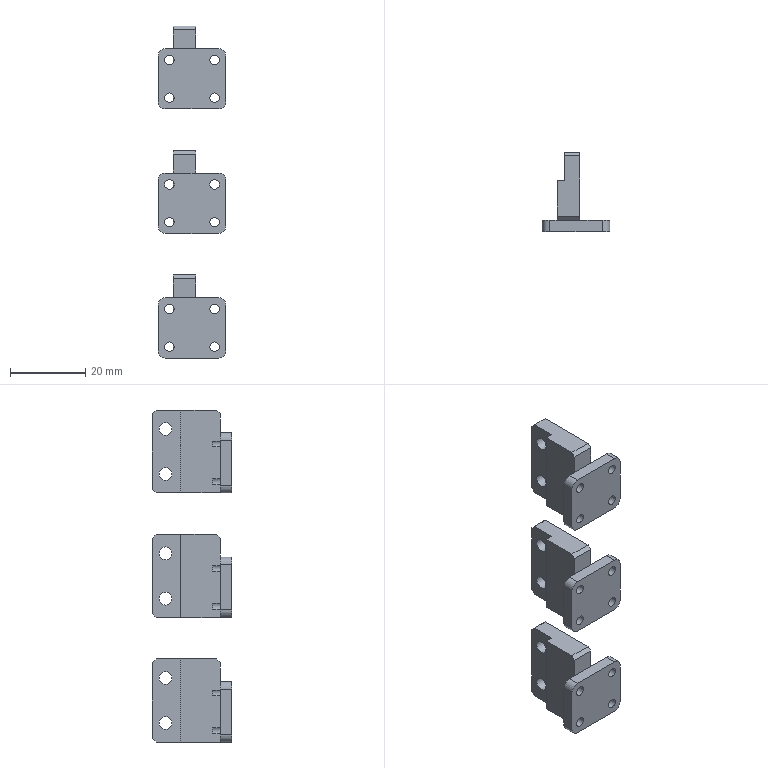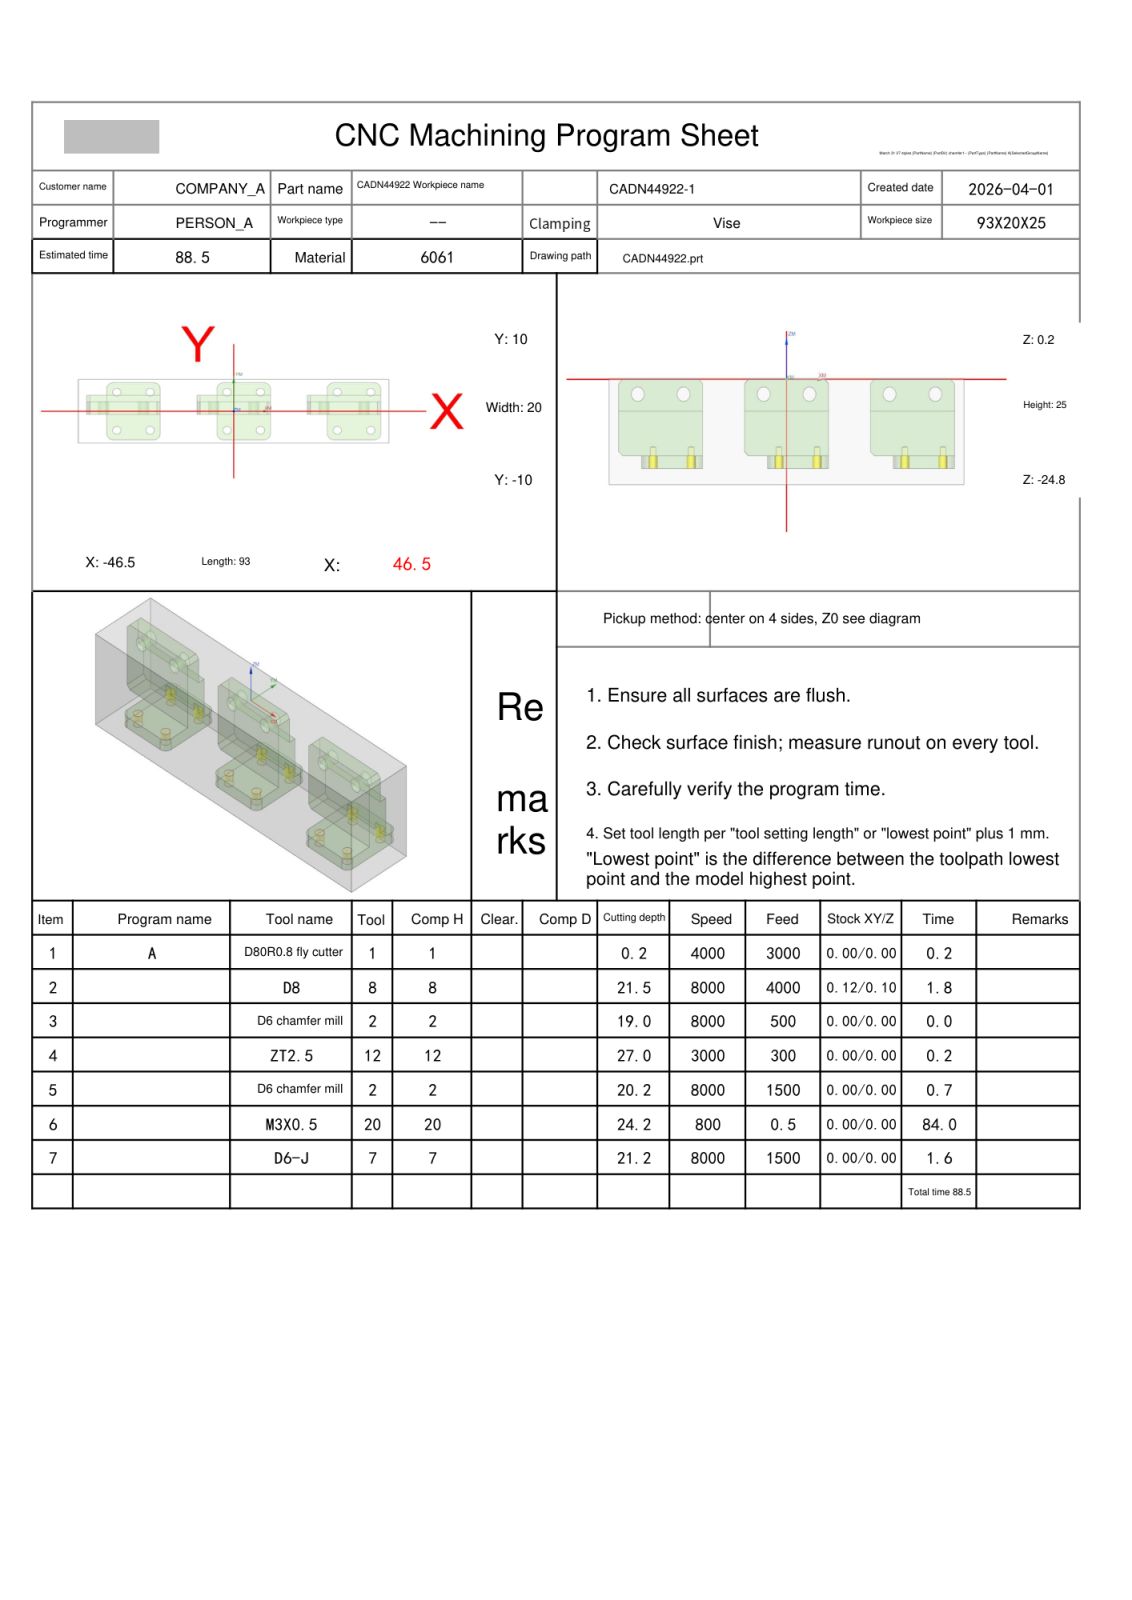NC program | NX | posted by the shop | part box 18 x 21 x 88 mm
Lines 3372 to 4142 of 4142:
N3 T02 M06
(D6 chamfer mill  D=6. R=0. H=02 ce=0.00 di=0.10)
G00 G90 G54 X-35. Y-6. M03 S8000
G43 H02 Z20.
M08
G98 G81 X-35. Y-6. Z-18.8 R-17. F500.
X-25.
X-2.
X8.
X31.
X41.
G80
G00 Z20.
G91 G28 Z0.0
M05
M09
G91 G28 Z0.0
M01
N4 T12 M06
(ZT2.5 D=2.5 DR_a=118 H=12)
G00 G90 G54 X-35. Y-6. M03 S3000
G43 H12 Z20.
M08
G98 G83 X-35. Y-6. Z-26.751 R-17. F300. Q2.
X-25.
X-2.
X8.
X31.
X41.
G80
G00 Z20.
G91 G28 Z0.0
M05
M09
G91 G28 Z0.0
M01
N5 T02 M06
(D6 chamfer mill  D=6. R=0. H=02 ce=0.00 di=0.10)
G00 G90 G54 X-35. Y-6. M03 S8000
G43 H02 Z20.
M08
G98 G81 X-35. Y-6. Z-19.75 R-15. F500.
X-25.
X-2.
X8.
X31.
X41.
G80
G00 Z20.
G00 G90 X-44.708 Y-3.9 M03 S6500
Z20.
Z-.2
G01 Z-1.7 F1500.
X-44.699 Y-3.832
X-44.7 Y-3.763
Y5.763
X-44.699 Y5.832
X-44.708 Y5.9
Z-.2
G00 Z20.
X-11.708 Y-3.9
Z-.2
G01 Z-1.7
X-11.699 Y-3.832
X-11.7 Y-3.763
Y5.763
X-11.699 Y5.832
X-11.708 Y5.9
Z-.2
G00 Z20.
X-21.292
Z-.2
G01 Z-1.7
X-21.301 Y5.832
X-21.3 Y5.763
Y-3.763
X-21.301 Y-3.832
X-21.292 Y-3.9
Z-.2
G00 Z20.
X21.292
Z-.2
G01 Z-1.7
X21.301 Y-3.832
X21.3 Y-3.763
Y5.763
X21.301 Y5.832
X21.292 Y5.9
Z-.2
G00 Z20.
X11.708
Z-.2
G01 Z-1.7
X11.699 Y5.832
X11.7 Y5.763
Y-3.763
X11.699 Y-3.832
X11.708 Y-3.9
Z-.2
G00 Z20.
X44.708 Y5.9
Z-.2
G01 Z-1.7
X44.699 Y5.832
X44.7 Y5.763
Y-3.763
X44.699 Y-3.832
X44.708 Y-3.9
Z-.2
G00 Z20.
G00 G90 X-43.604 Y4.689 M03 S6500
Z20.
Z2.
G01 Z-2. F1500.
X-43.351 Y4.765
X-43. Y4.8
X-23.
X-22.649 Y4.765
X-22.396 Y4.689
Z2.
G00 Y-2.689
G01 Z-2.
X-22.649 Y-2.765
X-23. Y-2.8
X-33.
X-43.
X-43.351 Y-2.765
X-43.604 Y-2.689
Z2.
G00 Z10.
X10.604
Z2.
G01 Z-2.
X10.351 Y-2.765
X10. Y-2.8
X-10.
X-10.351 Y-2.765
X-10.604 Y-2.689
Z2.
G00 Y4.689
G01 Z-2.
X-10.351 Y4.765
X-10. Y4.8
X0.0
X10.
X10.351 Y4.765
X10.604 Y4.689
Z2.
G00 Z10.
X43.604 Y-2.689
Z2.
G01 Z-2.
X43.351 Y-2.765
X43. Y-2.8
X23.
X22.649 Y-2.765
X22.396 Y-2.689
Z2.
G00 Y4.689
G01 Z-2.
X22.649 Y4.765
X23. Y4.8
X33.
X43.
X43.351 Y4.765
X43.604 Y4.689
Z2.
G00 Z10.
X20.059 Y5.65
Z-2.127
G01 Z-9.5
G03 X20.37 Y5.808 I-.745 J1.856
G01 X20.418 Y5.834
X20.441 Y5.883
X20.503 Y6.
G02 X22. Y6.8 I1.497 J-1.
G01 X23.375
X24.75
X27.5
X33.
X37.125
X39.875
X41.25
X44.
G02 X45.497 Y6. I0.0 J-1.8
G01 X45.559 Y5.883
X45.582 Y5.834
X45.63 Y5.808
G03 X45.941 Y5.65 I1.056 J1.698
G01 Z-2.127
G00 Z10.
X-12.941
Z-2.127
G01 Z-9.5
G03 X-12.63 Y5.808 I-.745 J1.856
G01 X-12.582 Y5.834
X-12.559 Y5.883
X-12.497 Y6.
G02 X-11. Y6.8 I1.497 J-1.
G01 X-9.625
X-8.25
X-5.5
X0.0
X4.125
X6.875
X8.25
X11.
G02 X12.497 Y6. I0.0 J-1.8
G01 X12.559 Y5.883
X12.582 Y5.834
X12.63 Y5.808
G03 X12.941 Y5.65 I1.056 J1.698
G01 Z-2.127
G00 Z10.
X-45.941
Z-2.127
G01 Z-9.5
G03 X-45.63 Y5.808 I-.745 J1.856
G01 X-45.582 Y5.834
X-45.559 Y5.883
X-45.497 Y6.
G02 X-44. Y6.8 I1.497 J-1.
G01 X-42.625
X-41.25
X-38.5
X-33.
X-28.875
X-26.125
X-24.75
X-22.
G02 X-20.503 Y6. I0.0 J-1.8
G01 X-20.441 Y5.883
X-20.418 Y5.834
X-20.37 Y5.808
G03 X-20.059 Y5.65 I1.056 J1.698
G01 Z-2.127
G00 Z10.
X-20.087 Y-3.573
Z-2.127
G01 Z-20.
X-20.148 Y-3.636
X-20.187 Y-3.716
X-20.206 Y-3.737
X-20.2 Y-3.766
Y-4.
Y-7.
G02 X-24. Y-10.8 I-3.8 J0.0
G01 X-31.5
X-33.
X-36.
G02 X-39.8 Y-7. I0.0 J3.8
G01 Y-4.281
X-39.805 Y-4.261
X-39.845 Y-4.204
Z-1.805
G00 Z10.
X-39.667 Y8.208
Z-9.31
G01 Z-20.
X-39.581 Y8.268
X-39.563 Y8.293
X-39.457 Y8.579
G02 X-36. Y10.8 I3.457 J-1.579
G01 X-24.
G02 X-20.354 Y8.071 I0.0 J-3.8
G01 X-20.296 Y7.806
X-20.289 Y7.757
X-20.254 Y7.723
G03 X-20.023 Y7.51 I1.332 J1.211
G01 Z-9.296
G00 Z10.
X12.913 Y-3.573
Z-2.127
G01 Z-20.
X12.852 Y-3.636
X12.813 Y-3.716
X12.794 Y-3.737
X12.8 Y-3.766
Y-7.
G02 X9. Y-10.8 I-3.8 J0.0
G01 X-3.
G02 X-6.8 Y-7. I0.0 J3.8
G01 Y-4.281
X-6.805 Y-4.261
X-6.845 Y-4.204
Z-1.805
G00 Z10.
X-6.667 Y8.208
Z-9.31
G01 Z-20.
X-6.581 Y8.268
X-6.563 Y8.293
X-6.457 Y8.579
G02 X-3. Y10.8 I3.457 J-1.579
G01 X9.
G02 X12.646 Y8.071 I0.0 J-3.8
G01 X12.704 Y7.806
X12.711 Y7.757
X12.746 Y7.723
G03 X12.977 Y7.51 I1.332 J1.211
G01 Z-9.296
G00 Z10.
X45.913 Y-3.573
Z-2.127
G01 Z-20.
X45.852 Y-3.636
X45.813 Y-3.716
X45.794 Y-3.737
X45.8 Y-3.766
Y-7.
G02 X42. Y-10.8 I-3.8 J0.0
G01 X30.
G02 X26.2 Y-7. I0.0 J3.8
G01 Y-4.281
X26.195 Y-4.261
X26.155 Y-4.204
Z-1.805
G00 Z10.
X26.333 Y8.208
Z-9.31
G01 Z-20.
X26.419 Y8.268
X26.437 Y8.293
X26.543 Y8.579
G02 X30. Y10.8 I3.457 J-1.579
G01 X42.
G02 X45.646 Y8.071 I0.0 J-3.8
G01 X45.704 Y7.806
X45.711 Y7.757
X45.746 Y7.723
G03 X45.977 Y7.51 I1.332 J1.211
G01 Z-9.296
G00 Z20.
G91 G28 Z0.0
M05
M09
G91 G28 Z0.0
M01
N6 T20 M06
(M3X0.5 D=2.5 DR_a=180 H=20)
G00 G90 G54 X-35. Y-6. M03 S800
G43 H20 Z20.
M08
G95
G98 G84 X-35. Y-6. Z-24. R-17. F.5 Q5.
X-25.
X-2.
X8.
X31.
X41.
G80
G94
G00 Z20.
G91 G28 Z0.0
M05
M09
G91 G28 Z0.0
M01
N7 T07 M06
(D6-J  D=6. R=0. H=07 ce=0.40 di=0.00)
G00 G90 G54 X-18.69 Y-10.2 M03 S7000
G43 H07 Z10.4
M08
Z-16.5
G01 Z-18. F1500.
G03 X-19.729 Y-9.6 I-1.039 J-.6
G01 X-39.919
G02 X-40.454 Y-9.273 I0.0 J.6
X-40.963 Y-7.605 I4.454 J2.273
G01 X-40.967 Y-7.54
G02 X-40.427 Y-7. I.54 J0.0
G01 X-19.54
G03 X-19. Y-6.46 I0.0 J.54
G01 Y-5.
G03 X-19.6 Y-4.4 I-.6 J0.0
G01 X-41.
G03 X-42.2 Y-5.6 I0.0 J-1.2
G01 Z-16.5
G00 Z-14.
X14.31 Y-10.2
Z-16.5
G01 Z-18.
G03 X13.271 Y-9.6 I-1.039 J-.6
G01 X-6.919
G02 X-7.454 Y-9.273 I0.0 J.6
X-7.963 Y-7.605 I4.454 J2.273
G01 X-7.967 Y-7.54
G02 X-7.427 Y-7. I.54 J0.0
G01 X13.46
G03 X14. Y-6.46 I0.0 J.54
G01 Y-5.
G03 X13.4 Y-4.4 I-.6 J0.0
G01 X-8.
G03 X-9.2 Y-5.6 I0.0 J-1.2
G01 Z-16.5
G00 Z-14.
X47.31 Y-10.2
Z-16.5
G01 Z-18.
G03 X46.271 Y-9.6 I-1.039 J-.6
G01 X26.08
G02 X25.547 Y-9.273 I0.0 J.6
X25.028 Y-7.531 I4.453 J2.273
G01 X25.026 Y-7.48
G02 X25.505 Y-7. I.48 J0.0
G01 X46.46
G03 X47. Y-6.46 I0.0 J.54
G01 Y-5.
G03 X46.4 Y-4.4 I-.6 J0.0
G01 X25.
G03 X23.8 Y-5.6 I0.0 J-1.2
G01 Z-16.5
G00 Z10.4
G00 G90 X21.083 Y6.995 M03 S8000
Z5.2
Z-4.25
G01 Z-5.25 F1000.
G41 D07
X21.106 Y6.796
G03 X22. Y6. I.894 J.104
G01 X44.
G02 X47. Y3. I0.0 J-3.
G01 Y-1.018
G02 X44. Y-4. I-3. J.018
G01 X22.
G02 X19. Y-1. I0.0 J3.
G01 Y3.
G02 X22. Y6. I3. J0.0
G03 X22.9 Y6.9 I0.0 J.9
G01 G40 Y7.1
Z-4.25
G00 Z5.2
X-44.917 Y6.995
Z-4.25
G01 Z-5.25
G41 D07
X-44.894 Y6.796
G03 X-44. Y6. I.894 J.104
G01 X-22.
G02 X-19. Y3. I0.0 J-3.
G01 Y-1.
X-19.001 Y-1.079
G02 X-22. Y-4. I-2.999 J.079
G01 X-44.
G02 X-47. Y-1. I0.0 J3.
G01 Y3.012
G02 X-44. Y6. I3. J-.012
G03 X-43.1 Y6.9 I0.0 J.9
G01 G40 Y7.1
Z-4.25
G00 Z5.2
X-11.917 Y6.995
Z-4.25
G01 Z-5.25
G41 D07
X-11.894 Y6.796
G03 X-11. Y6. I.894 J.104
G01 X11.
G02 X14. Y3. I0.0 J-3.
G01 Y-1.
X13.999 Y-1.078
G02 X11. Y-4. I-2.999 J.078
G01 X-11.
G02 X-14. Y-1. I0.0 J3.
G01 Y3.
G02 X-11. Y6. I3. J0.0
G03 X-10.1 Y6.9 I0.0 J.9
G01 G40 Y7.1
Z-4.25
G00 X-11.917 Y8.995
Z-9.5
G01 Z-10.5
G41 D07
X-11.894 Y8.796
G03 X-11. Y8. I.894 J.104
G01 X11.
G02 X13.999 Y5.077 I0.0 J-3.
G01 X14. Y5.
Y-1.
X13.999 Y-1.072
G02 X11. Y-4. I-2.999 J.072
G01 X-11.
G02 X-14. Y-1. I0.0 J3.
G01 Y5.
G02 X-11. Y8. I3. J0.0
G03 X-10.1 Y8.9 I0.0 J.9
G01 G40 Y9.1
Z-9.5
G00 Z3.
X-44.917 Y8.995
Z-9.5
G01 Z-10.5
G41 D07
X-44.894 Y8.796
G03 X-44. Y8. I.894 J.104
G01 X-22.
G02 X-19. Y5. I0.0 J-3.
G01 Y-1.
X-19.001 Y-1.079
G02 X-22. Y-4. I-2.999 J.079
G01 X-44.
G02 X-47. Y-1. I0.0 J3.
G01 Y5.
G02 X-44. Y8. I3. J0.0
G03 X-43.1 Y8.9 I0.0 J.9
G01 G40 Y9.1
Z-9.5
G00 X-44.917 Y8.995
Z-14.75
G01 Z-15.75
G41 D07
X-44.894 Y8.796
G03 X-44. Y8. I.894 J.104
G01 X-22.
G02 X-19. Y5. I0.0 J-3.
G01 Y-1.
X-19.001 Y-1.079
G02 X-22. Y-4. I-2.999 J.079
G01 X-44.
G02 X-47. Y-1. I0.0 J3.
G01 Y5.
G02 X-44. Y8. I3. J0.0
G03 X-43.1 Y8.9 I0.0 J.9
G01 G40 Y9.1
Z-14.75
G00 Z3.
X21.083 Y8.995
Z-9.5
G01 Z-10.5
G41 D07
X21.106 Y8.796
G03 X22. Y8. I.894 J.104
G01 X44.
G02 X47. Y5. I0.0 J-3.
G01 Y-1.014
G02 X44. Y-4. I-3. J.014
G01 X22.
G02 X19. Y-1. I0.0 J3.
G01 Y5.
G02 X22. Y8. I3. J0.0
G03 X22.9 Y8.9 I0.0 J.9
G01 G40 Y9.1
Z-9.5
G00 Z5.2
X-15.1 Y2.099
Z-6.5
G01 Z-7.5
G41 D07
X-14.9
G03 X-14. Y2.999 I0.0 J.9
G02 X-11. Y6. I3. J0.0
G01 X11.
G02 X14. Y3. I0.0 J-3.
G03 X14.9 Y2.099 I.9 J0.0
G01 G40 X15.1
Z-6.5
G00 Z5.2
X-48.1 Y2.104
Z-6.5
G01 Z-7.5
G41 D07
X-47.9
G03 X-47. Y2.999 I0.0 J.9
G01 Y3.031
G02 X-44. Y6. I3. J-.031
G01 X-22.
G02 X-19. Y3. I0.0 J-3.
G03 X-18.1 Y2.099 I.9 J0.0
G01 G40 X-17.9
Z-6.5
G00 Z5.2
X17.9 Y2.1
Z-6.5
G01 Z-7.5
G41 D07
X18.1
G03 X19. Y3. I0.0 J.9
G02 X22. Y6. I3. J0.0
G01 X44.
G02 X47. Y3. I0.0 J-3.
G03 X47.9 Y2.099 I.9 J0.0
G01 G40 X48.1
Z-6.5
G00 Z5.2
X21.083 Y8.995
Z-14.75
G01 Z-15.75
G41 D07
X21.106 Y8.796
G03 X22. Y8. I.894 J.104
G01 X44.
G02 X47. Y5. I0.0 J-3.
G01 Y-1.029
G02 X44. Y-4. I-3. J.029
G01 X22.
G02 X19. Y-1. I0.0 J3.
G01 Y5.
G02 X22. Y8. I3. J0.0
G03 X22.9 Y8.9 I0.0 J.9
G01 G40 Y9.1
Z-14.75
G00 Z5.2
X48.1 Y-.104
Z-17.
G01 Z-18.
G41 D07
X47.9
G03 X47. Y-.999 I0.0 J-.9
G01 Y-1.029
G02 X44. Y-4. I-3. J.029
G01 X25.
G03 X24.1 Y-4.9 I0.0 J-.9
G01 G40 Y-5.1
Z-17.
G00 Z5.2
X24.201 Y9.1
Z-17.
G01 Z-18.
G41 D07
Y8.9
G03 X25.101 Y8. I.9 J0.0
G01 X44.
G02 X47. Y5. I0.0 J-3.
G03 X47.9 Y4.099 I.9 J0.0
G01 G40 X48.1
Z-17.
G00 Z5.2
X-11.917 Y8.995
Z-14.75
G01 Z-15.75
G41 D07
X-11.894 Y8.796
G03 X-11. Y8. I.894 J.104
G01 X11.
G02 X14. Y5. I0.0 J-3.
G01 Y-1.
X13.999 Y-1.091
G02 X11. Y-4. I-2.999 J.091
G01 X-11.
G02 X-14. Y-1. I0.0 J3.
G01 Y5.
G02 X-11. Y8. I3. J0.0
G03 X-10.1 Y8.9 I0.0 J.9
G01 G40 Y9.1
Z-14.75
G00 Z5.2
X15.1 Y-.114
Z-17.
G01 Z-18.
G41 D07
X14.9
G03 X14. Y-1. I0.0 J-.9
G01 X13.999 Y-1.091
G02 X11. Y-4. I-2.999 J.091
G01 X-8.
G03 X-8.9 Y-4.9 I0.0 J-.9
G01 G40 Y-5.1
Z-17.
G00 Z5.2
X-8.799 Y9.1
Z-17.
G01 Z-18.
G41 D07
Y8.9
G03 X-7.899 Y8. I.9 J0.0
G01 X11.
G02 X14. Y5. I0.0 J-3.
G03 X14.9 Y4.1 I.9 J0.0
G01 G40 X15.1
Z-17.
G00 Z5.2
X-41.799 Y9.1
Z-17.
G01 Z-18.
G41 D07
Y8.9
G03 X-40.899 Y8. I.9 J0.0
G01 X-22.
G02 X-19. Y5. I0.0 J-3.
G03 X-18.1 Y4.099 I.9 J0.0
G01 G40 X-17.9
Z-17.
G00 Z5.2
Y-.111
Z-17.
G01 Z-18.
G41 D07
X-18.1
G03 X-19. Y-.999 I0.0 J-.9
G01 X-19.001 Y-1.079
G02 X-22. Y-4. I-2.999 J.079
G01 X-41.
G03 X-41.9 Y-4.9 I0.0 J-.9
G01 G40 Y-5.1
Z-17.
G00 Z5.2
X-3.913 Y13.031
Z-20.
G01 Z-21.
G41 D07
X-3.897 Y12.831
G03 X-3. Y12. I.897 J.069
G01 X9.
G02 X14. Y7. I0.0 J-5.
G01 Y-7.
G02 X9. Y-12. I-5. J0.0
G01 X-3.
G02 X-8. Y-7. I0.0 J5.
G01 Y-4.
X-11.
G02 X-14. Y-1. I0.0 J3.
G01 Y5.
G02 X-11. Y8. I3. J0.0
G01 X-7.899
G02 X-3. Y12. I4.899 J-1.
G03 X-2.1 Y12.9 I0.0 J.9
G01 G40 Y13.1
Z-20.
G00 Z-7.5
X-36.913 Y13.031
Z-20.
G01 Z-21.
G41 D07
X-36.897 Y12.831
G03 X-36. Y12. I.897 J.069
G01 X-24.
G02 X-19. Y7. I0.0 J-5.
G01 Y-7.
G02 X-24. Y-12. I-5. J0.0
G01 X-36.
G02 X-41. Y-7. I0.0 J5.
G01 Y-4.
X-44.
G02 X-47. Y-1. I0.0 J3.
G01 Y5.
G02 X-44. Y8. I3. J0.0
G01 X-40.899
G02 X-36. Y12. I4.899 J-1.
G03 X-35.1 Y12.9 I0.0 J.9
G01 G40 Y13.1
Z-20.
G00 Z-7.5
X29.087 Y13.031
Z-20.
G01 Z-21.
G41 D07
X29.103 Y12.831
G03 X30. Y12. I.897 J.069
G01 X42.
G02 X47. Y7. I0.0 J-5.
G01 Y-7.
G02 X42. Y-12. I-5. J0.0
G01 X30.
G02 X25. Y-7. I0.0 J5.
G01 Y-4.
X22.
G02 X19. Y-1. I0.0 J3.
G01 Y5.
G02 X22. Y8. I3. J0.0
G01 X25.101
G02 X30. Y12. I4.899 J-1.
G03 X30.9 Y12.9 I0.0 J.9
G01 G40 Y13.1
Z-20.
G00 Z5.2
M05
M09
G91 G28 Z0.0
G91 G28 Y0.0
M30
%